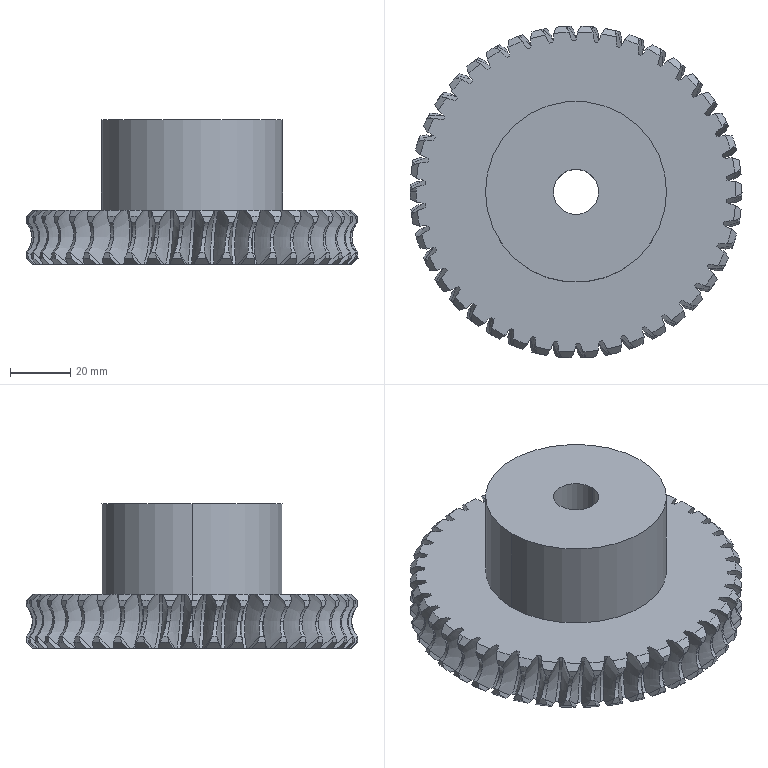Part | SolidWorks | features ICE 2, CirPattern 1, Helix 1, RefAxis 1, Revolution 1, SweepCut 1 | 1 solid | 475 faces | box 110.006 x 109.957 x 48 mm | volume 224193 mm3 | spline 210 | cylinder 90 | torus 86 | cone 86 | plane 3 | commonest cylinder face diameters 110.006 x86 15 x2 60 x2